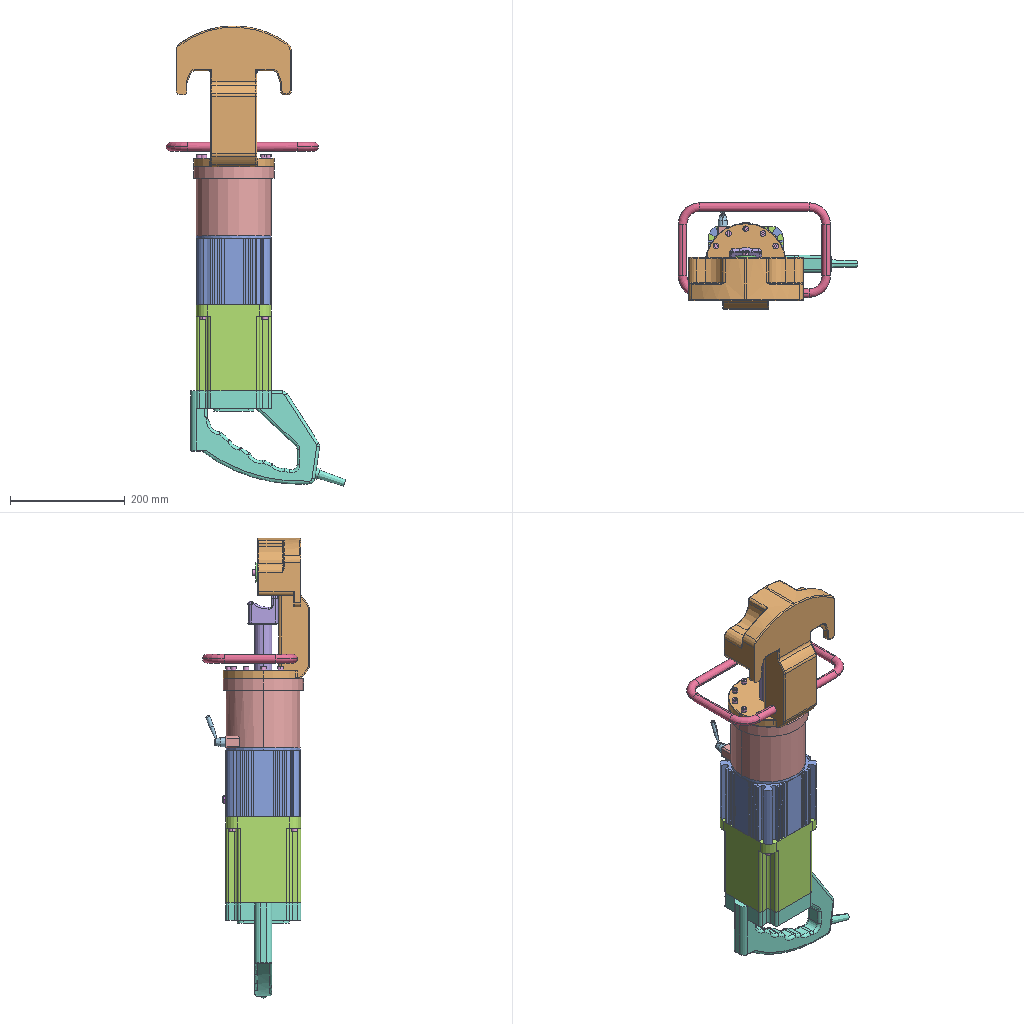Assembly | SolidWorks | 12 different items | 28 placed | box 312 x 186 x 800 mm
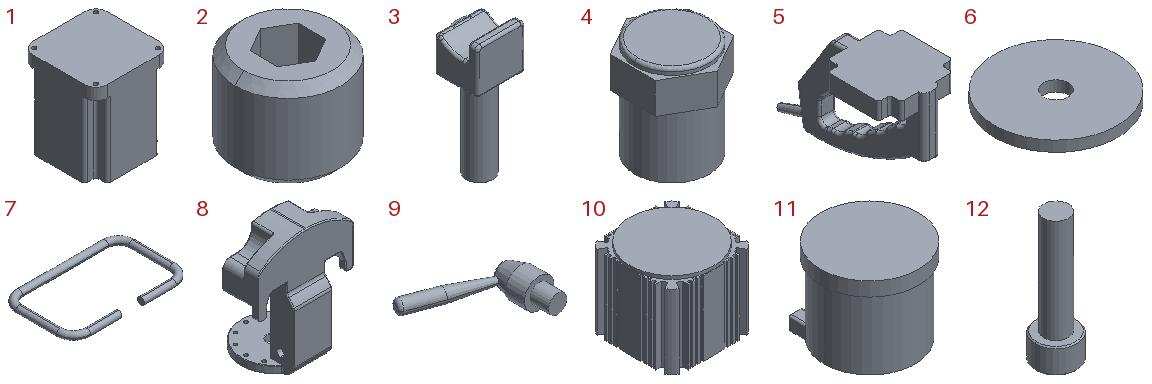Parts list (item | quantity | size | volume | features):
1 | x1 | 130 x 130 x 150 mm | 2314264 mm3 | features Fillet 3, CirPattern 2, ICE 2, Extrusion 1, RefAxis 1
2 | x1 | 12 x 12 x 10 mm | 968.16 mm3 | features Chamfer 1, Extrusion 1, ICE 1
3 | x1 | 55 x 52.5 x 150 mm | 171259 mm3 | features Fillet 9, ICE 4, Chamfer 1, Extrusion 1
4 | x1 | 12.619 x 14.572 x 16 mm | 1932 mm3 | features ICE 2, Extrusion 1, Fillet 1
5 | x1 | 130 x 269.835 x 165.306 mm | 953588 mm3 | features Fillet 14, ICE 12, CirPattern 2, Extrusion 1, MirrorPattern 1, RefAxis 1, Revolution 1
6 | x1 | 35 x 35 x 3 mm | 2771 mm3 | features Extrusion 1
7 | x1 | 265 x 165 x 15 mm | 123434 mm3 | features Sweep 1
8 | x1 | 200 x 150 x 245 mm | 1760406 mm3 | features Fillet 19, ICE 12, MirrorPattern 4, MoveFace 4, Chamfer 3, CirPattern 1, Extrusion 1
9 | x1 | 54.148 x 44.825 x 16 mm | 5470 mm3 | features Revolution 2, Fillet 1, ICE 1
10 | x1 | 130 x 130 x 120 mm | 1837022 mm3 | features ICE 3, CirPattern 1, Extrusion 1, Fillet 1, MirrorPattern 1
11 | x1 | 140 x 140 x 120 mm | 1639624 mm3 | features ICE 3, Extrusion 1, Fillet 1
12 | x17 | 10 x 10 x 31 mm | 1129 mm3 | features ICE 2, Chamfer 1, Extrusion 1
Mates (type | each side: item.copy, entity, surface, feature):
Concentric | 11.1 face cylinder Boss-Extrude1 | 10.1 face cylinder Cut-Extrude1
Coincident | 11.1 face plane Boss-Extrude4 | 10.1 face plane Boss-Extrude2
Coincident | 11.1 face plane Boss-Extrude1 | 10.1 face plane Boss-Extrude2
Concentric | 10.1 face cylinder Cut-Extrude1 | 1.1 select_type:24
Coincident | 10.1 face plane Boss-Extrude2 | 1.1 face plane Boss-Extrude1 | 2 times
Concentric | 1.1 face cylinder Cut-Extrude2 | 12.1 face cylinder Boss-Extrude2
Coincident | 1.1 face plane CirPattern1 | 12.1 face plane Boss-Extrude1
Coincident | 1.1 face plane Boss-Extrude1 | 5.1 face plane Boss-Extrude1 | 2 times
Coincident | 1.1 face plane Boss-Extrude1 | 5.1 face plane Cut-Extrude3
Coincident | 11.1 face plane Boss-Extrude2 | 8.1 face plane Boss-Extrude1
Concentric | 11.1 face cylinder Boss-Extrude2 | 8.1 face cylinder Boss-Extrude1
Parallel | 10.1 face plane Boss-Extrude2 | 8.1 face plane Boss-Extrude2
Parallel | 8.1 face plane Boss-Extrude2 | 3.1 face plane Boss-Extrude2
Concentric | 8.1 face cylinder Cut-Extrude7 | 6.1 face cylinder Boss-Extrude1
Coincident | 8.1 face plane Boss-Extrude3 | 6.1 face plane Boss-Extrude1
Concentric | 6.1 face cylinder Boss-Extrude1 | 12.2 face cylinder Boss-Extrude2
Coincident | 6.1 face plane Boss-Extrude1 | 12.2 face plane Boss-Extrude1
Concentric | 8.1 face cylinder Boss-Extrude1 | 3.1 face cylinder Boss-Extrude1
Concentric | 8.1 face cylinder CirPattern2 | 12.3 face cylinder Boss-Extrude2
Coincident | 8.1 face plane Boss-Extrude1 | 12.3 face plane Boss-Extrude1
Coincident | 8.1 face plane Boss-Extrude2 | 7.1 face plane Sweep1
Concentric | 11.1 face cylinder Cut-Extrude1 | 9.1 face cylinder Boss-Extrude1
Coincident | 11.1 face plane Boss-Extrude4 | 9.1 edge
Concentric | 10.1 face cylinder Cut-Extrude3 | 2.1 face cylinder Boss-Extrude1
DistanceDim | 10.1 face plane Boss-Extrude2 | 2.1 face plane Boss-Extrude1
Concentric | 10.1 face cylinder Cut-Extrude3 | 4.1 face cylinder Boss-Extrude1
Coincident | 10.1 face plane Boss-Extrude2 | 4.1 face plane Boss-Extrude2
LimitDistanceDim | 3.1 face plane Boss-Extrude2 | 8.1 face plane Boss-Extrude1
Parallel | 8.1 face plane Boss-Extrude1 | 7.1 plane
Concentric | 8.1 face cylinder Cut-Extrude10 | 7.1 face cylinder Sweep1